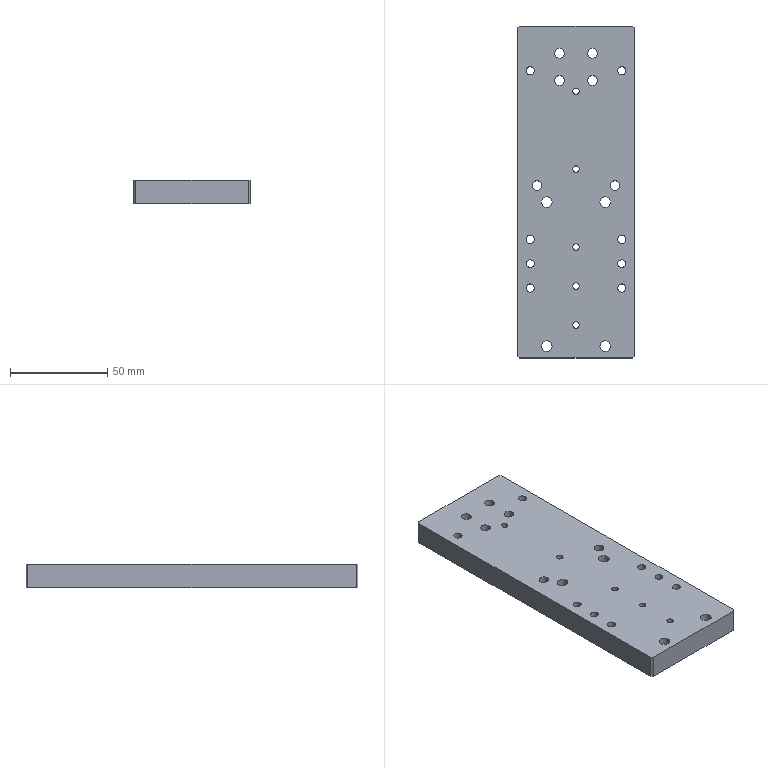Part | SolidWorks | features HoleWzd 6, Chamfer 1, Cut 1, Extrusion 1 | 1 solid | 74 faces | box 60 x 170.4 x 12 mm | volume 116995 mm3 | cylinder 58 | plane 16 | commonest cylinder face diameters 4.2 x12 5 x12 3.3 x10 5.5 x8 10 x8 4 x4